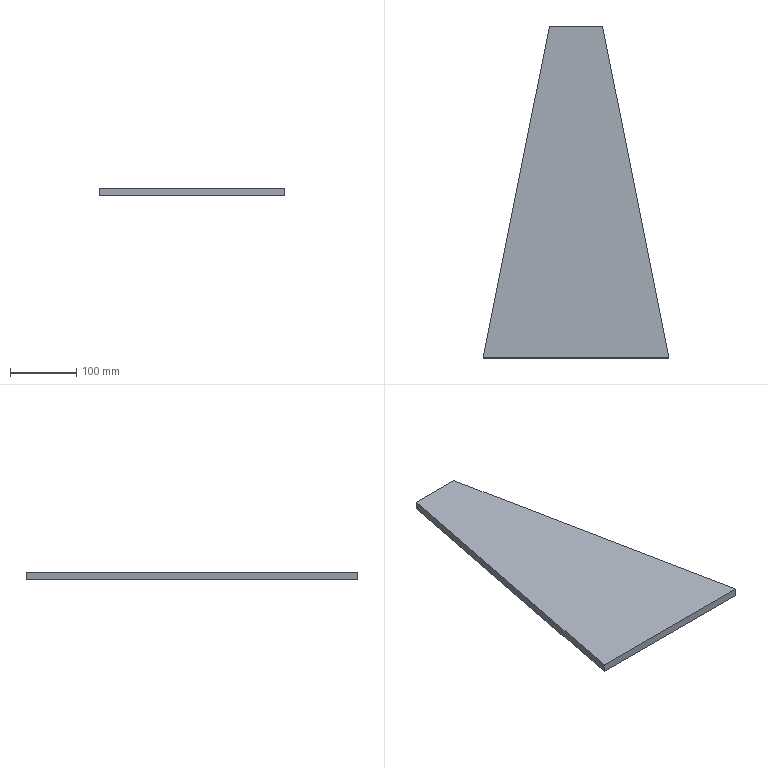Part | SolidWorks | features Extrusion 1, ICE 1 | 1 solid | 6 faces | box 280 x 500 x 12 mm | volume 1080000 mm3 | plane 6
STEP:
#1=CARTESIAN_POINT('',(-40.,250.,0.));
#2=VERTEX_POINT('',#1);
#3=CARTESIAN_POINT('',(-40.,250.,12.));
#4=VERTEX_POINT('',#3);
#5=CARTESIAN_POINT('',(-40.,250.,0.));
#6=DIRECTION('',(0.,0.,1.));
#7=VECTOR('',#6,1000.);
#8=LINE('',#5,#7);
#9=EDGE_CURVE('',#2,#4,#8,.T.);
#10=ORIENTED_EDGE('',*,*,#9,.T.);
#11=CARTESIAN_POINT('',(40.,250.,12.));
#12=VERTEX_POINT('',#11);
#13=CARTESIAN_POINT('',(140.,250.,12.));
#14=DIRECTION('',(-1.,0.,0.));
#15=VECTOR('',#14,1000.);
#16=LINE('',#13,#15);
#17=EDGE_CURVE('',#12,#4,#16,.T.);
#18=ORIENTED_EDGE('',*,*,#17,.F.);
#19=CARTESIAN_POINT('',(40.,250.,0.));
#20=VERTEX_POINT('',#19);
#21=CARTESIAN_POINT('',(40.,250.,0.));
#22=DIRECTION('',(0.,0.,1.));
#23=VECTOR('',#22,1000.);
#24=LINE('',#21,#23);
#25=EDGE_CURVE('',#20,#12,#24,.T.);
#26=ORIENTED_EDGE('',*,*,#25,.F.);
#27=CARTESIAN_POINT('',(140.,250.,0.));
#28=DIRECTION('',(-1.,0.,0.));
#29=VECTOR('',#28,1000.);
#30=LINE('',#27,#29);
#31=EDGE_CURVE('',#20,#2,#30,.T.);
#32=ORIENTED_EDGE('',*,*,#31,.T.);
#33=EDGE_LOOP('',(#10,#18,#26,#32));
#34=FACE_OUTER_BOUND('',#33,.T.);
#35=CARTESIAN_POINT('',(140.,250.,12.));
#36=DIRECTION('',(0.,-1.,0.));
#37=DIRECTION('',(1.,0.,0.));
#38=AXIS2_PLACEMENT_3D('',#35,#36,#37);
#39=PLANE('',#38);
#40=ADVANCED_FACE('',(#34),#39,.F.);
#41=CARTESIAN_POINT('',(-140.,-250.,12.));
#42=VERTEX_POINT('',#41);
#43=CARTESIAN_POINT('',(-140.,-250.,12.));
#44=DIRECTION('',(-0.1961,-0.9806,0.));
#45=VECTOR('',#44,1000.);
#46=LINE('',#43,#45);
#47=EDGE_CURVE('',#4,#42,#46,.T.);
#48=ORIENTED_EDGE('',*,*,#47,.T.);
#49=CARTESIAN_POINT('',(140.,-250.,12.));
#50=VERTEX_POINT('',#49);
#51=CARTESIAN_POINT('',(140.,-250.,12.));
#52=DIRECTION('',(1.,0.,0.));
#53=VECTOR('',#52,1000.);
#54=LINE('',#51,#53);
#55=EDGE_CURVE('',#42,#50,#54,.T.);
#56=ORIENTED_EDGE('',*,*,#55,.T.);
#57=CARTESIAN_POINT('',(40.,250.,12.));
#58=DIRECTION('',(-0.1961,0.9806,0.));
#59=VECTOR('',#58,1000.);
#60=LINE('',#57,#59);
#61=EDGE_CURVE('',#50,#12,#60,.T.);
#62=ORIENTED_EDGE('',*,*,#61,.T.);
#63=ORIENTED_EDGE('',*,*,#17,.T.);
#64=EDGE_LOOP('',(#48,#56,#62,#63));
#65=FACE_OUTER_BOUND('',#64,.T.);
#66=CARTESIAN_POINT('',(0.,0.,12.));
#67=DIRECTION('',(0.,0.,-1.));
#68=DIRECTION('',(-1.,0.,0.));
#69=AXIS2_PLACEMENT_3D('',#66,#67,#68);
#70=PLANE('',#69);
#71=ADVANCED_FACE('',(#65),#70,.F.);
#72=CARTESIAN_POINT('',(-140.,-250.,0.));
#73=VERTEX_POINT('',#72);
#74=CARTESIAN_POINT('',(140.,-250.,0.));
#75=VERTEX_POINT('',#74);
#76=CARTESIAN_POINT('',(140.,-250.,0.));
#77=DIRECTION('',(1.,0.,0.));
#78=VECTOR('',#77,1000.);
#79=LINE('',#76,#78);
#80=EDGE_CURVE('',#73,#75,#79,.T.);
#81=ORIENTED_EDGE('',*,*,#80,.F.);
#82=CARTESIAN_POINT('',(-140.,-250.,0.));
#83=DIRECTION('',(-0.1961,-0.9806,0.));
#84=VECTOR('',#83,1000.);
#85=LINE('',#82,#84);
#86=EDGE_CURVE('',#2,#73,#85,.T.);
#87=ORIENTED_EDGE('',*,*,#86,.F.);
#88=ORIENTED_EDGE('',*,*,#31,.F.);
#89=CARTESIAN_POINT('',(40.,250.,0.));
#90=DIRECTION('',(-0.1961,0.9806,0.));
#91=VECTOR('',#90,1000.);
#92=LINE('',#89,#91);
#93=EDGE_CURVE('',#75,#20,#92,.T.);
#94=ORIENTED_EDGE('',*,*,#93,.F.);
#95=EDGE_LOOP('',(#81,#87,#88,#94));
#96=FACE_OUTER_BOUND('',#95,.T.);
#97=CARTESIAN_POINT('',(0.,0.,0.));
#98=DIRECTION('',(0.,0.,-1.));
#99=DIRECTION('',(-1.,0.,0.));
#100=AXIS2_PLACEMENT_3D('',#97,#98,#99);
#101=PLANE('',#100);
#102=ADVANCED_FACE('',(#96),#101,.T.);
#103=ORIENTED_EDGE('',*,*,#80,.T.);
#104=CARTESIAN_POINT('',(140.,-250.,12.));
#105=DIRECTION('',(0.,0.,-1.));
#106=VECTOR('',#105,1000.);
#107=LINE('',#104,#106);
#108=EDGE_CURVE('',#50,#75,#107,.T.);
#109=ORIENTED_EDGE('',*,*,#108,.F.);
#110=ORIENTED_EDGE('',*,*,#55,.F.);
#111=CARTESIAN_POINT('',(-140.,-250.,12.));
#112=DIRECTION('',(0.,0.,-1.));
#113=VECTOR('',#112,1000.);
#114=LINE('',#111,#113);
#115=EDGE_CURVE('',#42,#73,#114,.T.);
#116=ORIENTED_EDGE('',*,*,#115,.T.);
#117=EDGE_LOOP('',(#103,#109,#110,#116));
#118=FACE_OUTER_BOUND('',#117,.T.);
#119=CARTESIAN_POINT('',(140.,-250.,12.));
#120=DIRECTION('',(0.,1.,0.));
#121=DIRECTION('',(-1.,0.,0.));
#122=AXIS2_PLACEMENT_3D('',#119,#120,#121);
#123=PLANE('',#122);
#124=ADVANCED_FACE('',(#118),#123,.F.);
#125=ORIENTED_EDGE('',*,*,#61,.F.);
#126=ORIENTED_EDGE('',*,*,#108,.T.);
#127=ORIENTED_EDGE('',*,*,#93,.T.);
#128=ORIENTED_EDGE('',*,*,#25,.T.);
#129=EDGE_LOOP('',(#125,#126,#127,#128));
#130=FACE_OUTER_BOUND('',#129,.T.);
#131=CARTESIAN_POINT('',(40.,250.,0.));
#132=DIRECTION('',(0.9806,0.1961,0.));
#133=DIRECTION('',(-0.1961,0.9806,0.));
#134=AXIS2_PLACEMENT_3D('',#131,#132,#133);
#135=PLANE('',#134);
#136=ADVANCED_FACE('',(#130),#135,.T.);
#137=ORIENTED_EDGE('',*,*,#47,.F.);
#138=ORIENTED_EDGE('',*,*,#9,.F.);
#139=ORIENTED_EDGE('',*,*,#86,.T.);
#140=ORIENTED_EDGE('',*,*,#115,.F.);
#141=EDGE_LOOP('',(#137,#138,#139,#140));
#142=FACE_OUTER_BOUND('',#141,.T.);
#143=CARTESIAN_POINT('',(-140.,-250.,0.));
#144=DIRECTION('',(-0.9806,0.1961,0.));
#145=DIRECTION('',(-0.1961,-0.9806,0.));
#146=AXIS2_PLACEMENT_3D('',#143,#144,#145);
#147=PLANE('',#146);
#148=ADVANCED_FACE('',(#142),#147,.T.);
#149=CLOSED_SHELL('',(#40,#71,#102,#124,#136,#148));
#150=MANIFOLD_SOLID_BREP('',#149);
#151=CARTESIAN_POINT('',(0.,0.,0.));
#152=DIRECTION('',(0.,0.,1.));
#153=DIRECTION('',(1.,0.,0.));
#154=AXIS2_PLACEMENT_3D('',#151,#152,#153);
#155=(LENGTH_UNIT()NAMED_UNIT(*)SI_UNIT(.MILLI.,.METRE.));
#156=UNCERTAINTY_MEASURE_WITH_UNIT(LENGTH_MEASURE(0.00001),#155,'','');
#157=(NAMED_UNIT(*)PLANE_ANGLE_UNIT()SI_UNIT($,.RADIAN.));
#158=(NAMED_UNIT(*)SI_UNIT($,.STERADIAN.)SOLID_ANGLE_UNIT());
#159=(GEOMETRIC_REPRESENTATION_CONTEXT(3)GLOBAL_UNCERTAINTY_ASSIGNED_CONTEXT((#156))GLOBAL_UNIT_ASSIGNED_CONTEXT((#155,#157,#158))REPRESENTATION_CONTEXT('',''));
#160=ADVANCED_BREP_SHAPE_REPRESENTATION('',(#150,#154),#159);